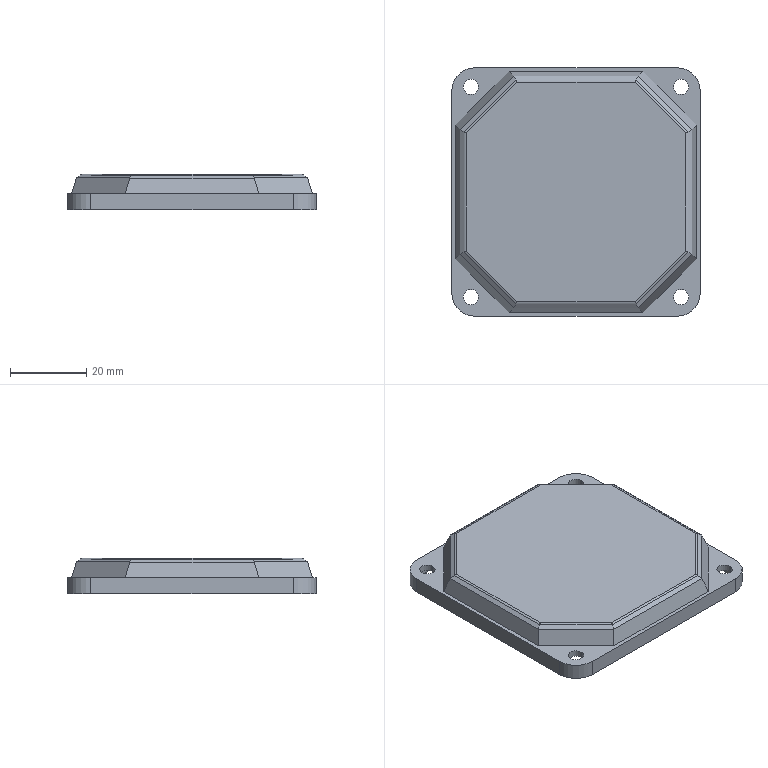Part | SolidWorks | features BaseBody 1 | 1 solid | 77 faces | box 65 x 65 x 9.2 mm | volume 10449 mm3 | plane 53 | cylinder 24 | commonest cylinder face diameters 2 x8 4 x8 9 x4 12 x4